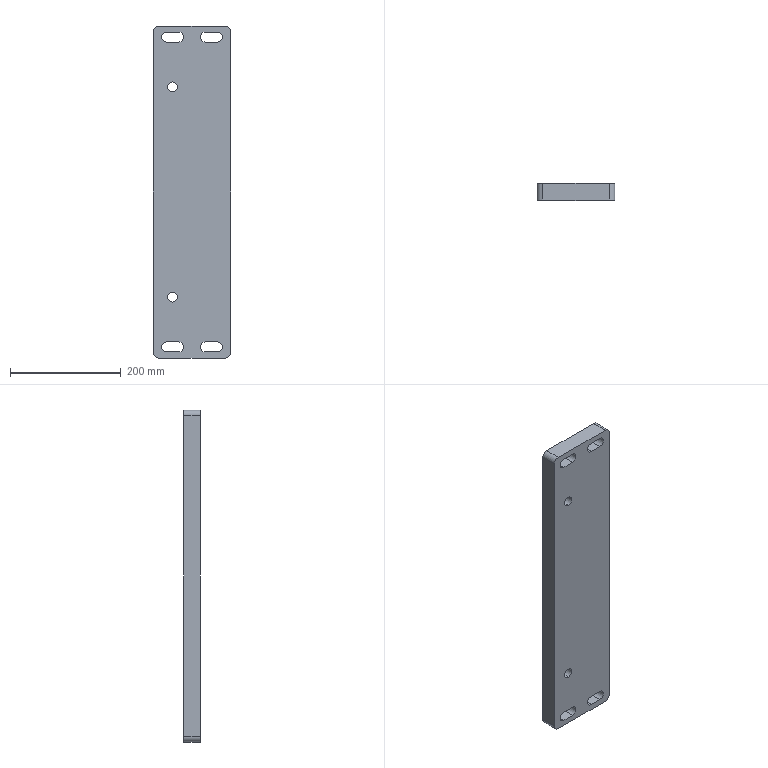Part | SolidWorks | features BaseBody 1 | 1 solid | 30 faces | box 140 x 30 x 600 mm | volume 2424100 mm3 | cylinder 16 | plane 14 | commonest cylinder face diameters 18 x12 20 x4
STEP:
#1=CARTESIAN_POINT('',(-35.,0.,181.));
#2=VERTEX_POINT('',#1);
#3=CARTESIAN_POINT('',(-35.,0.,199.));
#4=VERTEX_POINT('',#3);
#5=CARTESIAN_POINT('',(-35.,0.,190.));
#6=DIRECTION('',(0.,1.,0.));
#7=DIRECTION('',(0.,0.,1.));
#8=AXIS2_PLACEMENT_3D('',#5,#6,#7);
#9=CIRCLE('',#8,9.);
#10=EDGE_CURVE('',#2,#4,#9,.T.);
#11=ORIENTED_EDGE('',*,*,#10,.F.);
#12=CARTESIAN_POINT('',(-35.,30.,181.));
#13=VERTEX_POINT('',#12);
#14=CARTESIAN_POINT('',(-35.,30.,181.));
#15=DIRECTION('',(0.,1.,0.));
#16=VECTOR('',#15,1000.);
#17=LINE('',#14,#16);
#18=EDGE_CURVE('',#2,#13,#17,.T.);
#19=ORIENTED_EDGE('',*,*,#18,.T.);
#20=CARTESIAN_POINT('',(-35.,30.,199.));
#21=VERTEX_POINT('',#20);
#22=CARTESIAN_POINT('',(-35.,30.,190.));
#23=DIRECTION('',(0.,1.,0.));
#24=DIRECTION('',(0.,0.,1.));
#25=AXIS2_PLACEMENT_3D('',#22,#23,#24);
#26=CIRCLE('',#25,9.);
#27=EDGE_CURVE('',#13,#21,#26,.T.);
#28=ORIENTED_EDGE('',*,*,#27,.T.);
#29=CARTESIAN_POINT('',(-35.,30.,199.));
#30=DIRECTION('',(0.,1.,0.));
#31=VECTOR('',#30,1000.);
#32=LINE('',#29,#31);
#33=EDGE_CURVE('',#4,#21,#32,.T.);
#34=ORIENTED_EDGE('',*,*,#33,.F.);
#35=EDGE_LOOP('',(#11,#19,#28,#34));
#36=FACE_OUTER_BOUND('',#35,.T.);
#37=CARTESIAN_POINT('',(-35.,30.,190.));
#38=DIRECTION('',(0.,1.,0.));
#39=DIRECTION('',(0.,0.,1.));
#40=AXIS2_PLACEMENT_3D('',#37,#38,#39);
#41=CYLINDRICAL_SURFACE('',#40,9.);
#42=ADVANCED_FACE('',(#36),#41,.F.);
#43=CARTESIAN_POINT('',(-35.,0.,-199.));
#44=VERTEX_POINT('',#43);
#45=CARTESIAN_POINT('',(-35.,0.,-181.));
#46=VERTEX_POINT('',#45);
#47=CARTESIAN_POINT('',(-35.,0.,-190.));
#48=DIRECTION('',(0.,1.,0.));
#49=DIRECTION('',(0.,0.,1.));
#50=AXIS2_PLACEMENT_3D('',#47,#48,#49);
#51=CIRCLE('',#50,9.);
#52=EDGE_CURVE('',#44,#46,#51,.T.);
#53=ORIENTED_EDGE('',*,*,#52,.F.);
#54=CARTESIAN_POINT('',(-35.,30.,-199.));
#55=VERTEX_POINT('',#54);
#56=CARTESIAN_POINT('',(-35.,30.,-199.));
#57=DIRECTION('',(0.,1.,0.));
#58=VECTOR('',#57,1000.);
#59=LINE('',#56,#58);
#60=EDGE_CURVE('',#44,#55,#59,.T.);
#61=ORIENTED_EDGE('',*,*,#60,.T.);
#62=CARTESIAN_POINT('',(-35.,30.,-181.));
#63=VERTEX_POINT('',#62);
#64=CARTESIAN_POINT('',(-35.,30.,-190.));
#65=DIRECTION('',(0.,1.,0.));
#66=DIRECTION('',(0.,0.,1.));
#67=AXIS2_PLACEMENT_3D('',#64,#65,#66);
#68=CIRCLE('',#67,9.);
#69=EDGE_CURVE('',#55,#63,#68,.T.);
#70=ORIENTED_EDGE('',*,*,#69,.T.);
#71=CARTESIAN_POINT('',(-35.,30.,-181.));
#72=DIRECTION('',(0.,1.,0.));
#73=VECTOR('',#72,1000.);
#74=LINE('',#71,#73);
#75=EDGE_CURVE('',#46,#63,#74,.T.);
#76=ORIENTED_EDGE('',*,*,#75,.F.);
#77=EDGE_LOOP('',(#53,#61,#70,#76));
#78=FACE_OUTER_BOUND('',#77,.T.);
#79=CARTESIAN_POINT('',(-35.,30.,-190.));
#80=DIRECTION('',(0.,1.,0.));
#81=DIRECTION('',(0.,0.,1.));
#82=AXIS2_PLACEMENT_3D('',#79,#80,#81);
#83=CYLINDRICAL_SURFACE('',#82,9.);
#84=ADVANCED_FACE('',(#78),#83,.F.);
#85=CARTESIAN_POINT('',(70.,0.,290.));
#86=VERTEX_POINT('',#85);
#87=CARTESIAN_POINT('',(70.,0.,-290.));
#88=VERTEX_POINT('',#87);
#89=CARTESIAN_POINT('',(70.,0.,-300.));
#90=DIRECTION('',(0.,0.,-1.));
#91=VECTOR('',#90,1000.);
#92=LINE('',#89,#91);
#93=EDGE_CURVE('',#86,#88,#92,.T.);
#94=ORIENTED_EDGE('',*,*,#93,.T.);
#95=CARTESIAN_POINT('',(70.,30.,-290.));
#96=VERTEX_POINT('',#95);
#97=CARTESIAN_POINT('',(70.,30.,-290.));
#98=DIRECTION('',(0.,1.,0.));
#99=VECTOR('',#98,1000.);
#100=LINE('',#97,#99);
#101=EDGE_CURVE('',#88,#96,#100,.T.);
#102=ORIENTED_EDGE('',*,*,#101,.T.);
#103=CARTESIAN_POINT('',(70.,30.,290.));
#104=VERTEX_POINT('',#103);
#105=CARTESIAN_POINT('',(70.,30.,-300.));
#106=DIRECTION('',(0.,0.,-1.));
#107=VECTOR('',#106,1000.);
#108=LINE('',#105,#107);
#109=EDGE_CURVE('',#104,#96,#108,.T.);
#110=ORIENTED_EDGE('',*,*,#109,.F.);
#111=CARTESIAN_POINT('',(70.,30.,290.));
#112=DIRECTION('',(0.,-1.,0.));
#113=VECTOR('',#112,1000.);
#114=LINE('',#111,#113);
#115=EDGE_CURVE('',#104,#86,#114,.T.);
#116=ORIENTED_EDGE('',*,*,#115,.T.);
#117=EDGE_LOOP('',(#94,#102,#110,#116));
#118=FACE_OUTER_BOUND('',#117,.T.);
#119=CARTESIAN_POINT('',(70.,30.,-300.));
#120=DIRECTION('',(-1.,0.,0.));
#121=DIRECTION('',(0.,0.,1.));
#122=AXIS2_PLACEMENT_3D('',#119,#120,#121);
#123=PLANE('',#122);
#124=ADVANCED_FACE('',(#118),#123,.F.);
#125=CARTESIAN_POINT('',(60.,30.,-300.));
#126=VERTEX_POINT('',#125);
#127=CARTESIAN_POINT('',(-60.,30.,-300.));
#128=VERTEX_POINT('',#127);
#129=CARTESIAN_POINT('',(-70.,30.,-300.));
#130=DIRECTION('',(-1.,0.,0.));
#131=VECTOR('',#130,1000.);
#132=LINE('',#129,#131);
#133=EDGE_CURVE('',#126,#128,#132,.T.);
#134=ORIENTED_EDGE('',*,*,#133,.F.);
#135=CARTESIAN_POINT('',(60.,0.,-300.));
#136=VERTEX_POINT('',#135);
#137=CARTESIAN_POINT('',(60.,30.,-300.));
#138=DIRECTION('',(0.,-1.,0.));
#139=VECTOR('',#138,1000.);
#140=LINE('',#137,#139);
#141=EDGE_CURVE('',#126,#136,#140,.T.);
#142=ORIENTED_EDGE('',*,*,#141,.T.);
#143=CARTESIAN_POINT('',(-60.,0.,-300.));
#144=VERTEX_POINT('',#143);
#145=CARTESIAN_POINT('',(-70.,0.,-300.));
#146=DIRECTION('',(-1.,0.,0.));
#147=VECTOR('',#146,1000.);
#148=LINE('',#145,#147);
#149=EDGE_CURVE('',#136,#144,#148,.T.);
#150=ORIENTED_EDGE('',*,*,#149,.T.);
#151=CARTESIAN_POINT('',(-60.,30.,-300.));
#152=DIRECTION('',(0.,1.,0.));
#153=VECTOR('',#152,1000.);
#154=LINE('',#151,#153);
#155=EDGE_CURVE('',#144,#128,#154,.T.);
#156=ORIENTED_EDGE('',*,*,#155,.T.);
#157=EDGE_LOOP('',(#134,#142,#150,#156));
#158=FACE_OUTER_BOUND('',#157,.T.);
#159=CARTESIAN_POINT('',(-70.,30.,-300.));
#160=DIRECTION('',(0.,0.,1.));
#161=DIRECTION('',(1.,0.,0.));
#162=AXIS2_PLACEMENT_3D('',#159,#160,#161);
#163=PLANE('',#162);
#164=ADVANCED_FACE('',(#158),#163,.F.);
#165=CARTESIAN_POINT('',(-70.,30.,-290.));
#166=VERTEX_POINT('',#165);
#167=CARTESIAN_POINT('',(-70.,30.,290.));
#168=VERTEX_POINT('',#167);
#169=CARTESIAN_POINT('',(-70.,30.,-300.));
#170=DIRECTION('',(0.,0.,1.));
#171=VECTOR('',#170,1000.);
#172=LINE('',#169,#171);
#173=EDGE_CURVE('',#166,#168,#172,.T.);
#174=ORIENTED_EDGE('',*,*,#173,.F.);
#175=CARTESIAN_POINT('',(-70.,0.,-290.));
#176=VERTEX_POINT('',#175);
#177=CARTESIAN_POINT('',(-70.,30.,-290.));
#178=DIRECTION('',(0.,-1.,0.));
#179=VECTOR('',#178,1000.);
#180=LINE('',#177,#179);
#181=EDGE_CURVE('',#166,#176,#180,.T.);
#182=ORIENTED_EDGE('',*,*,#181,.T.);
#183=CARTESIAN_POINT('',(-70.,0.,290.));
#184=VERTEX_POINT('',#183);
#185=CARTESIAN_POINT('',(-70.,0.,-300.));
#186=DIRECTION('',(0.,0.,1.));
#187=VECTOR('',#186,1000.);
#188=LINE('',#185,#187);
#189=EDGE_CURVE('',#176,#184,#188,.T.);
#190=ORIENTED_EDGE('',*,*,#189,.T.);
#191=CARTESIAN_POINT('',(-70.,30.,290.));
#192=DIRECTION('',(0.,1.,0.));
#193=VECTOR('',#192,1000.);
#194=LINE('',#191,#193);
#195=EDGE_CURVE('',#184,#168,#194,.T.);
#196=ORIENTED_EDGE('',*,*,#195,.T.);
#197=EDGE_LOOP('',(#174,#182,#190,#196));
#198=FACE_OUTER_BOUND('',#197,.T.);
#199=CARTESIAN_POINT('',(-70.,30.,-300.));
#200=DIRECTION('',(1.,0.,0.));
#201=DIRECTION('',(0.,0.,-1.));
#202=AXIS2_PLACEMENT_3D('',#199,#200,#201);
#203=PLANE('',#202);
#204=ADVANCED_FACE('',(#198),#203,.F.);
#205=CARTESIAN_POINT('',(-60.,0.,300.));
#206=VERTEX_POINT('',#205);
#207=CARTESIAN_POINT('',(60.,0.,300.));
#208=VERTEX_POINT('',#207);
#209=CARTESIAN_POINT('',(-70.,0.,300.));
#210=DIRECTION('',(1.,0.,0.));
#211=VECTOR('',#210,1000.);
#212=LINE('',#209,#211);
#213=EDGE_CURVE('',#206,#208,#212,.T.);
#214=ORIENTED_EDGE('',*,*,#213,.T.);
#215=CARTESIAN_POINT('',(60.,30.,300.));
#216=VERTEX_POINT('',#215);
#217=CARTESIAN_POINT('',(60.,30.,300.));
#218=DIRECTION('',(0.,1.,0.));
#219=VECTOR('',#218,1000.);
#220=LINE('',#217,#219);
#221=EDGE_CURVE('',#208,#216,#220,.T.);
#222=ORIENTED_EDGE('',*,*,#221,.T.);
#223=CARTESIAN_POINT('',(-60.,30.,300.));
#224=VERTEX_POINT('',#223);
#225=CARTESIAN_POINT('',(-70.,30.,300.));
#226=DIRECTION('',(1.,0.,0.));
#227=VECTOR('',#226,1000.);
#228=LINE('',#225,#227);
#229=EDGE_CURVE('',#224,#216,#228,.T.);
#230=ORIENTED_EDGE('',*,*,#229,.F.);
#231=CARTESIAN_POINT('',(-60.,30.,300.));
#232=DIRECTION('',(0.,-1.,0.));
#233=VECTOR('',#232,1000.);
#234=LINE('',#231,#233);
#235=EDGE_CURVE('',#224,#206,#234,.T.);
#236=ORIENTED_EDGE('',*,*,#235,.T.);
#237=EDGE_LOOP('',(#214,#222,#230,#236));
#238=FACE_OUTER_BOUND('',#237,.T.);
#239=CARTESIAN_POINT('',(-70.,30.,300.));
#240=DIRECTION('',(0.,0.,-1.));
#241=DIRECTION('',(-1.,0.,0.));
#242=AXIS2_PLACEMENT_3D('',#239,#240,#241);
#243=PLANE('',#242);
#244=ADVANCED_FACE('',(#238),#243,.F.);
#245=CARTESIAN_POINT('',(24.,30.,271.));
#246=VERTEX_POINT('',#245);
#247=CARTESIAN_POINT('',(24.,30.,289.));
#248=VERTEX_POINT('',#247);
#249=CARTESIAN_POINT('',(24.,30.,280.));
#250=DIRECTION('',(0.,1.,0.));
#251=DIRECTION('',(0.,0.,1.));
#252=AXIS2_PLACEMENT_3D('',#249,#250,#251);
#253=CIRCLE('',#252,9.);
#254=EDGE_CURVE('',#246,#248,#253,.T.);
#255=ORIENTED_EDGE('',*,*,#254,.F.);
#256=CARTESIAN_POINT('',(46.,30.,271.));
#257=VERTEX_POINT('',#256);
#258=CARTESIAN_POINT('',(24.,30.,271.));
#259=DIRECTION('',(-1.,0.,0.));
#260=VECTOR('',#259,1000.);
#261=LINE('',#258,#260);
#262=EDGE_CURVE('',#257,#246,#261,.T.);
#263=ORIENTED_EDGE('',*,*,#262,.F.);
#264=CARTESIAN_POINT('',(46.,30.,289.));
#265=VERTEX_POINT('',#264);
#266=CARTESIAN_POINT('',(46.,30.,280.));
#267=DIRECTION('',(0.,1.,0.));
#268=DIRECTION('',(0.,0.,1.));
#269=AXIS2_PLACEMENT_3D('',#266,#267,#268);
#270=CIRCLE('',#269,9.);
#271=EDGE_CURVE('',#265,#257,#270,.T.);
#272=ORIENTED_EDGE('',*,*,#271,.F.);
#273=CARTESIAN_POINT('',(24.,30.,289.));
#274=DIRECTION('',(1.,0.,0.));
#275=VECTOR('',#274,1000.);
#276=LINE('',#273,#275);
#277=EDGE_CURVE('',#248,#265,#276,.T.);
#278=ORIENTED_EDGE('',*,*,#277,.F.);
#279=EDGE_LOOP('',(#255,#263,#272,#278));
#280=FACE_BOUND('',#279,.T.);
#281=CARTESIAN_POINT('',(-46.,30.,-289.));
#282=VERTEX_POINT('',#281);
#283=CARTESIAN_POINT('',(-46.,30.,-271.));
#284=VERTEX_POINT('',#283);
#285=CARTESIAN_POINT('',(-46.,30.,-280.));
#286=DIRECTION('',(0.,1.,0.));
#287=DIRECTION('',(0.,0.,-1.));
#288=AXIS2_PLACEMENT_3D('',#285,#286,#287);
#289=CIRCLE('',#288,9.);
#290=EDGE_CURVE('',#282,#284,#289,.T.);
#291=ORIENTED_EDGE('',*,*,#290,.F.);
#292=CARTESIAN_POINT('',(-24.,30.,-289.));
#293=VERTEX_POINT('',#292);
#294=CARTESIAN_POINT('',(-46.,30.,-289.));
#295=DIRECTION('',(-1.,0.,0.));
#296=VECTOR('',#295,1000.);
#297=LINE('',#294,#296);
#298=EDGE_CURVE('',#293,#282,#297,.T.);
#299=ORIENTED_EDGE('',*,*,#298,.F.);
#300=CARTESIAN_POINT('',(-24.,30.,-271.));
#301=VERTEX_POINT('',#300);
#302=CARTESIAN_POINT('',(-24.,30.,-280.));
#303=DIRECTION('',(0.,1.,0.));
#304=DIRECTION('',(0.,0.,-1.));
#305=AXIS2_PLACEMENT_3D('',#302,#303,#304);
#306=CIRCLE('',#305,9.);
#307=EDGE_CURVE('',#301,#293,#306,.T.);
#308=ORIENTED_EDGE('',*,*,#307,.F.);
#309=CARTESIAN_POINT('',(-46.,30.,-271.));
#310=DIRECTION('',(1.,0.,0.));
#311=VECTOR('',#310,1000.);
#312=LINE('',#309,#311);
#313=EDGE_CURVE('',#284,#301,#312,.T.);
#314=ORIENTED_EDGE('',*,*,#313,.F.);
#315=EDGE_LOOP('',(#291,#299,#308,#314));
#316=FACE_BOUND('',#315,.T.);
#317=CARTESIAN_POINT('',(24.,30.,-289.));
#318=VERTEX_POINT('',#317);
#319=CARTESIAN_POINT('',(24.,30.,-271.));
#320=VERTEX_POINT('',#319);
#321=CARTESIAN_POINT('',(24.,30.,-280.));
#322=DIRECTION('',(0.,1.,0.));
#323=DIRECTION('',(0.,0.,-1.));
#324=AXIS2_PLACEMENT_3D('',#321,#322,#323);
#325=CIRCLE('',#324,9.);
#326=EDGE_CURVE('',#318,#320,#325,.T.);
#327=ORIENTED_EDGE('',*,*,#326,.F.);
#328=CARTESIAN_POINT('',(46.,30.,-289.));
#329=VERTEX_POINT('',#328);
#330=CARTESIAN_POINT('',(24.,30.,-289.));
#331=DIRECTION('',(-1.,0.,0.));
#332=VECTOR('',#331,1000.);
#333=LINE('',#330,#332);
#334=EDGE_CURVE('',#329,#318,#333,.T.);
#335=ORIENTED_EDGE('',*,*,#334,.F.);
#336=CARTESIAN_POINT('',(46.,30.,-271.));
#337=VERTEX_POINT('',#336);
#338=CARTESIAN_POINT('',(46.,30.,-280.));
#339=DIRECTION('',(0.,1.,0.));
#340=DIRECTION('',(0.,0.,-1.));
#341=AXIS2_PLACEMENT_3D('',#338,#339,#340);
#342=CIRCLE('',#341,9.);
#343=EDGE_CURVE('',#337,#329,#342,.T.);
#344=ORIENTED_EDGE('',*,*,#343,.F.);
#345=CARTESIAN_POINT('',(24.,30.,-271.));
#346=DIRECTION('',(1.,0.,0.));
#347=VECTOR('',#346,1000.);
#348=LINE('',#345,#347);
#349=EDGE_CURVE('',#320,#337,#348,.T.);
#350=ORIENTED_EDGE('',*,*,#349,.F.);
#351=EDGE_LOOP('',(#327,#335,#344,#350));
#352=FACE_BOUND('',#351,.T.);
#353=CARTESIAN_POINT('',(-46.,30.,271.));
#354=VERTEX_POINT('',#353);
#355=CARTESIAN_POINT('',(-46.,30.,289.));
#356=VERTEX_POINT('',#355);
#357=CARTESIAN_POINT('',(-46.,30.,280.));
#358=DIRECTION('',(0.,1.,0.));
#359=DIRECTION('',(0.,0.,1.));
#360=AXIS2_PLACEMENT_3D('',#357,#358,#359);
#361=CIRCLE('',#360,9.);
#362=EDGE_CURVE('',#354,#356,#361,.T.);
#363=ORIENTED_EDGE('',*,*,#362,.F.);
#364=CARTESIAN_POINT('',(-24.,30.,271.));
#365=VERTEX_POINT('',#364);
#366=CARTESIAN_POINT('',(-46.,30.,271.));
#367=DIRECTION('',(-1.,0.,0.));
#368=VECTOR('',#367,1000.);
#369=LINE('',#366,#368);
#370=EDGE_CURVE('',#365,#354,#369,.T.);
#371=ORIENTED_EDGE('',*,*,#370,.F.);
#372=CARTESIAN_POINT('',(-24.,30.,289.));
#373=VERTEX_POINT('',#372);
#374=CARTESIAN_POINT('',(-24.,30.,280.));
#375=DIRECTION('',(0.,1.,0.));
#376=DIRECTION('',(0.,0.,1.));
#377=AXIS2_PLACEMENT_3D('',#374,#375,#376);
#378=CIRCLE('',#377,9.);
#379=EDGE_CURVE('',#373,#365,#378,.T.);
#380=ORIENTED_EDGE('',*,*,#379,.F.);
#381=CARTESIAN_POINT('',(-46.,30.,289.));
#382=DIRECTION('',(1.,0.,0.));
#383=VECTOR('',#382,1000.);
#384=LINE('',#381,#383);
#385=EDGE_CURVE('',#356,#373,#384,.T.);
#386=ORIENTED_EDGE('',*,*,#385,.F.);
#387=EDGE_LOOP('',(#363,#371,#380,#386));
#388=FACE_BOUND('',#387,.T.);
#389=CARTESIAN_POINT('',(-35.,30.,190.));
#390=DIRECTION('',(0.,1.,0.));
#391=DIRECTION('',(0.,0.,1.));
#392=AXIS2_PLACEMENT_3D('',#389,#390,#391);
#393=CIRCLE('',#392,9.);
#394=EDGE_CURVE('',#21,#13,#393,.T.);
#395=ORIENTED_EDGE('',*,*,#394,.F.);
#396=ORIENTED_EDGE('',*,*,#27,.F.);
#397=EDGE_LOOP('',(#395,#396));
#398=FACE_BOUND('',#397,.T.);
#399=CARTESIAN_POINT('',(-35.,30.,-190.));
#400=DIRECTION('',(0.,1.,0.));
#401=DIRECTION('',(0.,0.,1.));
#402=AXIS2_PLACEMENT_3D('',#399,#400,#401);
#403=CIRCLE('',#402,9.);
#404=EDGE_CURVE('',#63,#55,#403,.T.);
#405=ORIENTED_EDGE('',*,*,#404,.F.);
#406=ORIENTED_EDGE('',*,*,#69,.F.);
#407=EDGE_LOOP('',(#405,#406));
#408=FACE_BOUND('',#407,.T.);
#409=ORIENTED_EDGE('',*,*,#109,.T.);
#410=CARTESIAN_POINT('',(60.,30.,-290.));
#411=DIRECTION('',(0.,1.,0.));
#412=DIRECTION('',(0.,0.,1.));
#413=AXIS2_PLACEMENT_3D('',#410,#411,#412);
#414=CIRCLE('',#413,10.);
#415=EDGE_CURVE('',#96,#126,#414,.T.);
#416=ORIENTED_EDGE('',*,*,#415,.T.);
#417=ORIENTED_EDGE('',*,*,#133,.T.);
#418=CARTESIAN_POINT('',(-60.,30.,-290.));
#419=DIRECTION('',(0.,1.,0.));
#420=DIRECTION('',(0.,0.,1.));
#421=AXIS2_PLACEMENT_3D('',#418,#419,#420);
#422=CIRCLE('',#421,10.);
#423=EDGE_CURVE('',#128,#166,#422,.T.);
#424=ORIENTED_EDGE('',*,*,#423,.T.);
#425=ORIENTED_EDGE('',*,*,#173,.T.);
#426=CARTESIAN_POINT('',(-60.,30.,290.));
#427=DIRECTION('',(0.,1.,0.));
#428=DIRECTION('',(0.,0.,1.));
#429=AXIS2_PLACEMENT_3D('',#426,#427,#428);
#430=CIRCLE('',#429,10.);
#431=EDGE_CURVE('',#168,#224,#430,.T.);
#432=ORIENTED_EDGE('',*,*,#431,.T.);
#433=ORIENTED_EDGE('',*,*,#229,.T.);
#434=CARTESIAN_POINT('',(60.,30.,290.));
#435=DIRECTION('',(0.,1.,0.));
#436=DIRECTION('',(0.,0.,1.));
#437=AXIS2_PLACEMENT_3D('',#434,#435,#436);
#438=CIRCLE('',#437,10.);
#439=EDGE_CURVE('',#216,#104,#438,.T.);
#440=ORIENTED_EDGE('',*,*,#439,.T.);
#441=EDGE_LOOP('',(#409,#416,#417,#424,#425,#432,#433,#440));
#442=FACE_OUTER_BOUND('',#441,.T.);
#443=CARTESIAN_POINT('',(0.,30.,0.));
#444=DIRECTION('',(0.,1.,0.));
#445=DIRECTION('',(0.,0.,1.));
#446=AXIS2_PLACEMENT_3D('',#443,#444,#445);
#447=PLANE('',#446);
#448=ADVANCED_FACE('',(#280,#316,#352,#388,#398,#408,#442),#447,.T.);
#449=CARTESIAN_POINT('',(46.,0.,271.));
#450=VERTEX_POINT('',#449);
#451=CARTESIAN_POINT('',(24.,0.,271.));
#452=VERTEX_POINT('',#451);
#453=CARTESIAN_POINT('',(24.,0.,271.));
#454=DIRECTION('',(-1.,0.,0.));
#455=VECTOR('',#454,1000.);
#456=LINE('',#453,#455);
#457=EDGE_CURVE('',#450,#452,#456,.T.);
#458=ORIENTED_EDGE('',*,*,#457,.T.);
#459=CARTESIAN_POINT('',(24.,0.,289.));
#460=VERTEX_POINT('',#459);
#461=CARTESIAN_POINT('',(24.,0.,280.));
#462=DIRECTION('',(0.,1.,0.));
#463=DIRECTION('',(0.,0.,1.));
#464=AXIS2_PLACEMENT_3D('',#461,#462,#463);
#465=CIRCLE('',#464,9.);
#466=EDGE_CURVE('',#452,#460,#465,.T.);
#467=ORIENTED_EDGE('',*,*,#466,.T.);
#468=CARTESIAN_POINT('',(46.,0.,289.));
#469=VERTEX_POINT('',#468);
#470=CARTESIAN_POINT('',(24.,0.,289.));
#471=DIRECTION('',(1.,0.,0.));
#472=VECTOR('',#471,1000.);
#473=LINE('',#470,#472);
#474=EDGE_CURVE('',#460,#469,#473,.T.);
#475=ORIENTED_EDGE('',*,*,#474,.T.);
#476=CARTESIAN_POINT('',(46.,0.,280.));
#477=DIRECTION('',(0.,1.,0.));
#478=DIRECTION('',(0.,0.,1.));
#479=AXIS2_PLACEMENT_3D('',#476,#477,#478);
#480=CIRCLE('',#479,9.);
#481=EDGE_CURVE('',#469,#450,#480,.T.);
#482=ORIENTED_EDGE('',*,*,#481,.T.);
#483=EDGE_LOOP('',(#458,#467,#475,#482));
#484=FACE_BOUND('',#483,.T.);
#485=CARTESIAN_POINT('',(-24.,0.,-289.));
#486=VERTEX_POINT('',#485);
#487=CARTESIAN_POINT('',(-46.,0.,-289.));
#488=VERTEX_POINT('',#487);
#489=CARTESIAN_POINT('',(-46.,0.,-289.));
#490=DIRECTION('',(-1.,0.,0.));
#491=VECTOR('',#490,1000.);
#492=LINE('',#489,#491);
#493=EDGE_CURVE('',#486,#488,#492,.T.);
#494=ORIENTED_EDGE('',*,*,#493,.T.);
#495=CARTESIAN_POINT('',(-46.,0.,-271.));
#496=VERTEX_POINT('',#495);
#497=CARTESIAN_POINT('',(-46.,0.,-280.));
#498=DIRECTION('',(0.,1.,0.));
#499=DIRECTION('',(0.,0.,-1.));
#500=AXIS2_PLACEMENT_3D('',#497,#498,#499);
#501=CIRCLE('',#500,9.);
#502=EDGE_CURVE('',#488,#496,#501,.T.);
#503=ORIENTED_EDGE('',*,*,#502,.T.);
#504=CARTESIAN_POINT('',(-24.,0.,-271.));
#505=VERTEX_POINT('',#504);
#506=CARTESIAN_POINT('',(-46.,0.,-271.));
#507=DIRECTION('',(1.,0.,0.));
#508=VECTOR('',#507,1000.);
#509=LINE('',#506,#508);
#510=EDGE_CURVE('',#496,#505,#509,.T.);
#511=ORIENTED_EDGE('',*,*,#510,.T.);
#512=CARTESIAN_POINT('',(-24.,0.,-280.));
#513=DIRECTION('',(0.,1.,0.));
#514=DIRECTION('',(0.,0.,-1.));
#515=AXIS2_PLACEMENT_3D('',#512,#513,#514);
#516=CIRCLE('',#515,9.);
#517=EDGE_CURVE('',#505,#486,#516,.T.);
#518=ORIENTED_EDGE('',*,*,#517,.T.);
#519=EDGE_LOOP('',(#494,#503,#511,#518));
#520=FACE_BOUND('',#519,.T.);
#521=CARTESIAN_POINT('',(46.,0.,-289.));
#522=VERTEX_POINT('',#521);
#523=CARTESIAN_POINT('',(24.,0.,-289.));
#524=VERTEX_POINT('',#523);
#525=CARTESIAN_POINT('',(24.,0.,-289.));
#526=DIRECTION('',(-1.,0.,0.));
#527=VECTOR('',#526,1000.);
#528=LINE('',#525,#527);
#529=EDGE_CURVE('',#522,#524,#528,.T.);
#530=ORIENTED_EDGE('',*,*,#529,.T.);
#531=CARTESIAN_POINT('',(24.,0.,-271.));
#532=VERTEX_POINT('',#531);
#533=CARTESIAN_POINT('',(24.,0.,-280.));
#534=DIRECTION('',(0.,1.,0.));
#535=DIRECTION('',(0.,0.,-1.));
#536=AXIS2_PLACEMENT_3D('',#533,#534,#535);
#537=CIRCLE('',#536,9.);
#538=EDGE_CURVE('',#524,#532,#537,.T.);
#539=ORIENTED_EDGE('',*,*,#538,.T.);
#540=CARTESIAN_POINT('',(46.,0.,-271.));
#541=VERTEX_POINT('',#540);
#542=CARTESIAN_POINT('',(24.,0.,-271.));
#543=DIRECTION('',(1.,0.,0.));
#544=VECTOR('',#543,1000.);
#545=LINE('',#542,#544);
#546=EDGE_CURVE('',#532,#541,#545,.T.);
#547=ORIENTED_EDGE('',*,*,#546,.T.);
#548=CARTESIAN_POINT('',(46.,0.,-280.));
#549=DIRECTION('',(0.,1.,0.));
#550=DIRECTION('',(0.,0.,-1.));
#551=AXIS2_PLACEMENT_3D('',#548,#549,#550);
#552=CIRCLE('',#551,9.);
#553=EDGE_CURVE('',#541,#522,#552,.T.);
#554=ORIENTED_EDGE('',*,*,#553,.T.);
#555=EDGE_LOOP('',(#530,#539,#547,#554));
#556=FACE_BOUND('',#555,.T.);
#557=CARTESIAN_POINT('',(-24.,0.,271.));
#558=VERTEX_POINT('',#557);
#559=CARTESIAN_POINT('',(-46.,0.,271.));
#560=VERTEX_POINT('',#559);
#561=CARTESIAN_POINT('',(-46.,0.,271.));
#562=DIRECTION('',(-1.,0.,0.));
#563=VECTOR('',#562,1000.);
#564=LINE('',#561,#563);
#565=EDGE_CURVE('',#558,#560,#564,.T.);
#566=ORIENTED_EDGE('',*,*,#565,.T.);
#567=CARTESIAN_POINT('',(-46.,0.,289.));
#568=VERTEX_POINT('',#567);
#569=CARTESIAN_POINT('',(-46.,0.,280.));
#570=DIRECTION('',(0.,1.,0.));
#571=DIRECTION('',(0.,0.,1.));
#572=AXIS2_PLACEMENT_3D('',#569,#570,#571);
#573=CIRCLE('',#572,9.);
#574=EDGE_CURVE('',#560,#568,#573,.T.);
#575=ORIENTED_EDGE('',*,*,#574,.T.);
#576=CARTESIAN_POINT('',(-24.,0.,289.));
#577=VERTEX_POINT('',#576);
#578=CARTESIAN_POINT('',(-46.,0.,289.));
#579=DIRECTION('',(1.,0.,0.));
#580=VECTOR('',#579,1000.);
#581=LINE('',#578,#580);
#582=EDGE_CURVE('',#568,#577,#581,.T.);
#583=ORIENTED_EDGE('',*,*,#582,.T.);
#584=CARTESIAN_POINT('',(-24.,0.,280.));
#585=DIRECTION('',(0.,1.,0.));
#586=DIRECTION('',(0.,0.,1.));
#587=AXIS2_PLACEMENT_3D('',#584,#585,#586);
#588=CIRCLE('',#587,9.);
#589=EDGE_CURVE('',#577,#558,#588,.T.);
#590=ORIENTED_EDGE('',*,*,#589,.T.);
#591=EDGE_LOOP('',(#566,#575,#583,#590));
#592=FACE_BOUND('',#591,.T.);
#593=CARTESIAN_POINT('',(-35.,0.,190.));
#594=DIRECTION('',(0.,1.,0.));
#595=DIRECTION('',(0.,0.,1.));
#596=AXIS2_PLACEMENT_3D('',#593,#594,#595);
#597=CIRCLE('',#596,9.);
#598=EDGE_CURVE('',#4,#2,#597,.T.);
#599=ORIENTED_EDGE('',*,*,#598,.T.);
#600=ORIENTED_EDGE('',*,*,#10,.T.);
#601=EDGE_LOOP('',(#599,#600));
#602=FACE_BOUND('',#601,.T.);
#603=CARTESIAN_POINT('',(-35.,0.,-190.));
#604=DIRECTION('',(0.,1.,0.));
#605=DIRECTION('',(0.,0.,1.));
#606=AXIS2_PLACEMENT_3D('',#603,#604,#605);
#607=CIRCLE('',#606,9.);
#608=EDGE_CURVE('',#46,#44,#607,.T.);
#609=ORIENTED_EDGE('',*,*,#608,.T.);
#610=ORIENTED_EDGE('',*,*,#52,.T.);
#611=EDGE_LOOP('',(#609,#610));
#612=FACE_BOUND('',#611,.T.);
#613=ORIENTED_EDGE('',*,*,#149,.F.);
#614=CARTESIAN_POINT('',(60.,0.,-290.));
#615=DIRECTION('',(0.,-1.,0.));
#616=DIRECTION('',(0.,0.,1.));
#617=AXIS2_PLACEMENT_3D('',#614,#615,#616);
#618=CIRCLE('',#617,10.);
#619=EDGE_CURVE('',#136,#88,#618,.T.);
#620=ORIENTED_EDGE('',*,*,#619,.T.);
#621=ORIENTED_EDGE('',*,*,#93,.F.);
#622=CARTESIAN_POINT('',(60.,0.,290.));
#623=DIRECTION('',(0.,-1.,0.));
#624=DIRECTION('',(0.,0.,1.));
#625=AXIS2_PLACEMENT_3D('',#622,#623,#624);
#626=CIRCLE('',#625,10.);
#627=EDGE_CURVE('',#86,#208,#626,.T.);
#628=ORIENTED_EDGE('',*,*,#627,.T.);
#629=ORIENTED_EDGE('',*,*,#213,.F.);
#630=CARTESIAN_POINT('',(-60.,0.,290.));
#631=DIRECTION('',(0.,-1.,0.));
#632=DIRECTION('',(0.,0.,1.));
#633=AXIS2_PLACEMENT_3D('',#630,#631,#632);
#634=CIRCLE('',#633,10.);
#635=EDGE_CURVE('',#206,#184,#634,.T.);
#636=ORIENTED_EDGE('',*,*,#635,.T.);
#637=ORIENTED_EDGE('',*,*,#189,.F.);
#638=CARTESIAN_POINT('',(-60.,0.,-290.));
#639=DIRECTION('',(0.,-1.,0.));
#640=DIRECTION('',(0.,0.,1.));
#641=AXIS2_PLACEMENT_3D('',#638,#639,#640);
#642=CIRCLE('',#641,10.);
#643=EDGE_CURVE('',#176,#144,#642,.T.);
#644=ORIENTED_EDGE('',*,*,#643,.T.);
#645=EDGE_LOOP('',(#613,#620,#621,#628,#629,#636,#637,#644));
#646=FACE_OUTER_BOUND('',#645,.T.);
#647=CARTESIAN_POINT('',(0.,0.,0.));
#648=DIRECTION('',(0.,1.,0.));
#649=DIRECTION('',(0.,0.,1.));
#650=AXIS2_PLACEMENT_3D('',#647,#648,#649);
#651=PLANE('',#650);
#652=ADVANCED_FACE('',(#484,#520,#556,#592,#602,#612,#646),#651,.F.);
#653=ORIENTED_EDGE('',*,*,#60,.F.);
#654=ORIENTED_EDGE('',*,*,#608,.F.);
#655=ORIENTED_EDGE('',*,*,#75,.T.);
#656=ORIENTED_EDGE('',*,*,#404,.T.);
#657=EDGE_LOOP('',(#653,#654,#655,#656));
#658=FACE_OUTER_BOUND('',#657,.T.);
#659=CARTESIAN_POINT('',(-35.,30.,-190.));
#660=DIRECTION('',(0.,1.,0.));
#661=DIRECTION('',(0.,0.,1.));
#662=AXIS2_PLACEMENT_3D('',#659,#660,#661);
#663=CYLINDRICAL_SURFACE('',#662,9.);
#664=ADVANCED_FACE('',(#658),#663,.F.);
#665=ORIENTED_EDGE('',*,*,#18,.F.);
#666=ORIENTED_EDGE('',*,*,#598,.F.);
#667=ORIENTED_EDGE('',*,*,#33,.T.);
#668=ORIENTED_EDGE('',*,*,#394,.T.);
#669=EDGE_LOOP('',(#665,#666,#667,#668));
#670=FACE_OUTER_BOUND('',#669,.T.);
#671=CARTESIAN_POINT('',(-35.,30.,190.));
#672=DIRECTION('',(0.,1.,0.));
#673=DIRECTION('',(0.,0.,1.));
#674=AXIS2_PLACEMENT_3D('',#671,#672,#673);
#675=CYLINDRICAL_SURFACE('',#674,9.);
#676=ADVANCED_FACE('',(#670),#675,.F.);
#677=ORIENTED_EDGE('',*,*,#415,.F.);
#678=ORIENTED_EDGE('',*,*,#101,.F.);
#679=ORIENTED_EDGE('',*,*,#619,.F.);
#680=ORIENTED_EDGE('',*,*,#141,.F.);
#681=EDGE_LOOP('',(#677,#678,#679,#680));
#682=FACE_OUTER_BOUND('',#681,.T.);
#683=CARTESIAN_POINT('',(60.,30.,-290.));
#684=DIRECTION('',(0.,-1.,0.));
#685=DIRECTION('',(0.,0.,-1.));
#686=AXIS2_PLACEMENT_3D('',#683,#684,#685);
#687=CYLINDRICAL_SURFACE('',#686,10.);
#688=ADVANCED_FACE('',(#682),#687,.T.);
#689=ORIENTED_EDGE('',*,*,#423,.F.);
#690=ORIENTED_EDGE('',*,*,#155,.F.);
#691=ORIENTED_EDGE('',*,*,#643,.F.);
#692=ORIENTED_EDGE('',*,*,#181,.F.);
#693=EDGE_LOOP('',(#689,#690,#691,#692));
#694=FACE_OUTER_BOUND('',#693,.T.);
#695=CARTESIAN_POINT('',(-60.,30.,-290.));
#696=DIRECTION('',(0.,-1.,0.));
#697=DIRECTION('',(0.,0.,-1.));
#698=AXIS2_PLACEMENT_3D('',#695,#696,#697);
#699=CYLINDRICAL_SURFACE('',#698,10.);
#700=ADVANCED_FACE('',(#694),#699,.T.);
#701=ORIENTED_EDGE('',*,*,#439,.F.);
#702=ORIENTED_EDGE('',*,*,#221,.F.);
#703=ORIENTED_EDGE('',*,*,#627,.F.);
#704=ORIENTED_EDGE('',*,*,#115,.F.);
#705=EDGE_LOOP('',(#701,#702,#703,#704));
#706=FACE_OUTER_BOUND('',#705,.T.);
#707=CARTESIAN_POINT('',(60.,30.,290.));
#708=DIRECTION('',(0.,-1.,0.));
#709=DIRECTION('',(0.,0.,-1.));
#710=AXIS2_PLACEMENT_3D('',#707,#708,#709);
#711=CYLINDRICAL_SURFACE('',#710,10.);
#712=ADVANCED_FACE('',(#706),#711,.T.);
#713=ORIENTED_EDGE('',*,*,#431,.F.);
#714=ORIENTED_EDGE('',*,*,#195,.F.);
#715=ORIENTED_EDGE('',*,*,#635,.F.);
#716=ORIENTED_EDGE('',*,*,#235,.F.);
#717=EDGE_LOOP('',(#713,#714,#715,#716));
#718=FACE_OUTER_BOUND('',#717,.T.);
#719=CARTESIAN_POINT('',(-60.,30.,290.));
#720=DIRECTION('',(0.,-1.,0.));
#721=DIRECTION('',(0.,0.,-1.));
#722=AXIS2_PLACEMENT_3D('',#719,#720,#721);
#723=CYLINDRICAL_SURFACE('',#722,10.);
#724=ADVANCED_FACE('',(#718),#723,.T.);
#725=ORIENTED_EDGE('',*,*,#362,.T.);
#726=CARTESIAN_POINT('',(-46.,0.,289.));
#727=DIRECTION('',(0.,1.,0.));
#728=VECTOR('',#727,1000.);
#729=LINE('',#726,#728);
#730=EDGE_CURVE('',#568,#356,#729,.T.);
#731=ORIENTED_EDGE('',*,*,#730,.F.);
#732=ORIENTED_EDGE('',*,*,#574,.F.);
#733=CARTESIAN_POINT('',(-46.,0.,271.));
#734=DIRECTION('',(0.,1.,0.));
#735=VECTOR('',#734,1000.);
#736=LINE('',#733,#735);
#737=EDGE_CURVE('',#560,#354,#736,.T.);
#738=ORIENTED_EDGE('',*,*,#737,.T.);
#739=EDGE_LOOP('',(#725,#731,#732,#738));
#740=FACE_OUTER_BOUND('',#739,.T.);
#741=CARTESIAN_POINT('',(-46.,0.,280.));
#742=DIRECTION('',(0.,1.,0.));
#743=DIRECTION('',(0.,0.,1.));
#744=AXIS2_PLACEMENT_3D('',#741,#742,#743);
#745=CYLINDRICAL_SURFACE('',#744,9.);
#746=ADVANCED_FACE('',(#740),#745,.F.);
#747=ORIENTED_EDGE('',*,*,#370,.T.);
#748=ORIENTED_EDGE('',*,*,#737,.F.);
#749=ORIENTED_EDGE('',*,*,#565,.F.);
#750=CARTESIAN_POINT('',(-24.,0.,271.));
#751=DIRECTION('',(0.,1.,0.));
#752=VECTOR('',#751,1000.);
#753=LINE('',#750,#752);
#754=EDGE_CURVE('',#558,#365,#753,.T.);
#755=ORIENTED_EDGE('',*,*,#754,.T.);
#756=EDGE_LOOP('',(#747,#748,#749,#755));
#757=FACE_OUTER_BOUND('',#756,.T.);
#758=CARTESIAN_POINT('',(-46.,0.,271.));
#759=DIRECTION('',(0.,0.,-1.));
#760=DIRECTION('',(-1.,0.,0.));
#761=AXIS2_PLACEMENT_3D('',#758,#759,#760);
#762=PLANE('',#761);
#763=ADVANCED_FACE('',(#757),#762,.F.);
#764=ORIENTED_EDGE('',*,*,#379,.T.);
#765=ORIENTED_EDGE('',*,*,#754,.F.);
#766=ORIENTED_EDGE('',*,*,#589,.F.);
#767=CARTESIAN_POINT('',(-24.,0.,289.));
#768=DIRECTION('',(0.,1.,0.));
#769=VECTOR('',#768,1000.);
#770=LINE('',#767,#769);
#771=EDGE_CURVE('',#577,#373,#770,.T.);
#772=ORIENTED_EDGE('',*,*,#771,.T.);
#773=EDGE_LOOP('',(#764,#765,#766,#772));
#774=FACE_OUTER_BOUND('',#773,.T.);
#775=CARTESIAN_POINT('',(-24.,0.,280.));
#776=DIRECTION('',(0.,1.,0.));
#777=DIRECTION('',(0.,0.,1.));
#778=AXIS2_PLACEMENT_3D('',#775,#776,#777);
#779=CYLINDRICAL_SURFACE('',#778,9.);
#780=ADVANCED_FACE('',(#774),#779,.F.);
#781=ORIENTED_EDGE('',*,*,#385,.T.);
#782=ORIENTED_EDGE('',*,*,#771,.F.);
#783=ORIENTED_EDGE('',*,*,#582,.F.);
#784=ORIENTED_EDGE('',*,*,#730,.T.);
#785=EDGE_LOOP('',(#781,#782,#783,#784));
#786=FACE_OUTER_BOUND('',#785,.T.);
#787=CARTESIAN_POINT('',(-46.,0.,289.));
#788=DIRECTION('',(0.,0.,1.));
#789=DIRECTION('',(1.,0.,0.));
#790=AXIS2_PLACEMENT_3D('',#787,#788,#789);
#791=PLANE('',#790);
#792=ADVANCED_FACE('',(#786),#791,.F.);
#793=ORIENTED_EDGE('',*,*,#326,.T.);
#794=CARTESIAN_POINT('',(24.,0.,-271.));
#795=DIRECTION('',(0.,1.,0.));
#796=VECTOR('',#795,1000.);
#797=LINE('',#794,#796);
#798=EDGE_CURVE('',#532,#320,#797,.T.);
#799=ORIENTED_EDGE('',*,*,#798,.F.);
#800=ORIENTED_EDGE('',*,*,#538,.F.);
#801=CARTESIAN_POINT('',(24.,0.,-289.));
#802=DIRECTION('',(0.,1.,0.));
#803=VECTOR('',#802,1000.);
#804=LINE('',#801,#803);
#805=EDGE_CURVE('',#524,#318,#804,.T.);
#806=ORIENTED_EDGE('',*,*,#805,.T.);
#807=EDGE_LOOP('',(#793,#799,#800,#806));
#808=FACE_OUTER_BOUND('',#807,.T.);
#809=CARTESIAN_POINT('',(24.,0.,-280.));
#810=DIRECTION('',(0.,1.,0.));
#811=DIRECTION('',(0.,0.,1.));
#812=AXIS2_PLACEMENT_3D('',#809,#810,#811);
#813=CYLINDRICAL_SURFACE('',#812,9.);
#814=ADVANCED_FACE('',(#808),#813,.F.);
#815=ORIENTED_EDGE('',*,*,#334,.T.);
#816=ORIENTED_EDGE('',*,*,#805,.F.);
#817=ORIENTED_EDGE('',*,*,#529,.F.);
#818=CARTESIAN_POINT('',(46.,0.,-289.));
#819=DIRECTION('',(0.,1.,0.));
#820=VECTOR('',#819,1000.);
#821=LINE('',#818,#820);
#822=EDGE_CURVE('',#522,#329,#821,.T.);
#823=ORIENTED_EDGE('',*,*,#822,.T.);
#824=EDGE_LOOP('',(#815,#816,#817,#823));
#825=FACE_OUTER_BOUND('',#824,.T.);
#826=CARTESIAN_POINT('',(24.,0.,-289.));
#827=DIRECTION('',(0.,0.,-1.));
#828=DIRECTION('',(-1.,0.,0.));
#829=AXIS2_PLACEMENT_3D('',#826,#827,#828);
#830=PLANE('',#829);
#831=ADVANCED_FACE('',(#825),#830,.F.);
#832=ORIENTED_EDGE('',*,*,#343,.T.);
#833=ORIENTED_EDGE('',*,*,#822,.F.);
#834=ORIENTED_EDGE('',*,*,#553,.F.);
#835=CARTESIAN_POINT('',(46.,0.,-271.));
#836=DIRECTION('',(0.,1.,0.));
#837=VECTOR('',#836,1000.);
#838=LINE('',#835,#837);
#839=EDGE_CURVE('',#541,#337,#838,.T.);
#840=ORIENTED_EDGE('',*,*,#839,.T.);
#841=EDGE_LOOP('',(#832,#833,#834,#840));
#842=FACE_OUTER_BOUND('',#841,.T.);
#843=CARTESIAN_POINT('',(46.,0.,-280.));
#844=DIRECTION('',(0.,1.,0.));
#845=DIRECTION('',(0.,0.,1.));
#846=AXIS2_PLACEMENT_3D('',#843,#844,#845);
#847=CYLINDRICAL_SURFACE('',#846,9.);
#848=ADVANCED_FACE('',(#842),#847,.F.);
#849=ORIENTED_EDGE('',*,*,#349,.T.);
#850=ORIENTED_EDGE('',*,*,#839,.F.);
#851=ORIENTED_EDGE('',*,*,#546,.F.);
#852=ORIENTED_EDGE('',*,*,#798,.T.);
#853=EDGE_LOOP('',(#849,#850,#851,#852));
#854=FACE_OUTER_BOUND('',#853,.T.);
#855=CARTESIAN_POINT('',(24.,0.,-271.));
#856=DIRECTION('',(0.,0.,1.));
#857=DIRECTION('',(1.,0.,0.));
#858=AXIS2_PLACEMENT_3D('',#855,#856,#857);
#859=PLANE('',#858);
#860=ADVANCED_FACE('',(#854),#859,.F.);
#861=ORIENTED_EDGE('',*,*,#290,.T.);
#862=CARTESIAN_POINT('',(-46.,0.,-271.));
#863=DIRECTION('',(0.,1.,0.));
#864=VECTOR('',#863,1000.);
#865=LINE('',#862,#864);
#866=EDGE_CURVE('',#496,#284,#865,.T.);
#867=ORIENTED_EDGE('',*,*,#866,.F.);
#868=ORIENTED_EDGE('',*,*,#502,.F.);
#869=CARTESIAN_POINT('',(-46.,0.,-289.));
#870=DIRECTION('',(0.,1.,0.));
#871=VECTOR('',#870,1000.);
#872=LINE('',#869,#871);
#873=EDGE_CURVE('',#488,#282,#872,.T.);
#874=ORIENTED_EDGE('',*,*,#873,.T.);
#875=EDGE_LOOP('',(#861,#867,#868,#874));
#876=FACE_OUTER_BOUND('',#875,.T.);
#877=CARTESIAN_POINT('',(-46.,0.,-280.));
#878=DIRECTION('',(0.,1.,0.));
#879=DIRECTION('',(0.,0.,1.));
#880=AXIS2_PLACEMENT_3D('',#877,#878,#879);
#881=CYLINDRICAL_SURFACE('',#880,9.);
#882=ADVANCED_FACE('',(#876),#881,.F.);
#883=ORIENTED_EDGE('',*,*,#298,.T.);
#884=ORIENTED_EDGE('',*,*,#873,.F.);
#885=ORIENTED_EDGE('',*,*,#493,.F.);
#886=CARTESIAN_POINT('',(-24.,0.,-289.));
#887=DIRECTION('',(0.,1.,0.));
#888=VECTOR('',#887,1000.);
#889=LINE('',#886,#888);
#890=EDGE_CURVE('',#486,#293,#889,.T.);
#891=ORIENTED_EDGE('',*,*,#890,.T.);
#892=EDGE_LOOP('',(#883,#884,#885,#891));
#893=FACE_OUTER_BOUND('',#892,.T.);
#894=CARTESIAN_POINT('',(-46.,0.,-289.));
#895=DIRECTION('',(0.,0.,-1.));
#896=DIRECTION('',(-1.,0.,0.));
#897=AXIS2_PLACEMENT_3D('',#894,#895,#896);
#898=PLANE('',#897);
#899=ADVANCED_FACE('',(#893),#898,.F.);
#900=ORIENTED_EDGE('',*,*,#307,.T.);
#901=ORIENTED_EDGE('',*,*,#890,.F.);
#902=ORIENTED_EDGE('',*,*,#517,.F.);
#903=CARTESIAN_POINT('',(-24.,0.,-271.));
#904=DIRECTION('',(0.,1.,0.));
#905=VECTOR('',#904,1000.);
#906=LINE('',#903,#905);
#907=EDGE_CURVE('',#505,#301,#906,.T.);
#908=ORIENTED_EDGE('',*,*,#907,.T.);
#909=EDGE_LOOP('',(#900,#901,#902,#908));
#910=FACE_OUTER_BOUND('',#909,.T.);
#911=CARTESIAN_POINT('',(-24.,0.,-280.));
#912=DIRECTION('',(0.,1.,0.));
#913=DIRECTION('',(0.,0.,1.));
#914=AXIS2_PLACEMENT_3D('',#911,#912,#913);
#915=CYLINDRICAL_SURFACE('',#914,9.);
#916=ADVANCED_FACE('',(#910),#915,.F.);
#917=ORIENTED_EDGE('',*,*,#313,.T.);
#918=ORIENTED_EDGE('',*,*,#907,.F.);
#919=ORIENTED_EDGE('',*,*,#510,.F.);
#920=ORIENTED_EDGE('',*,*,#866,.T.);
#921=EDGE_LOOP('',(#917,#918,#919,#920));
#922=FACE_OUTER_BOUND('',#921,.T.);
#923=CARTESIAN_POINT('',(-46.,0.,-271.));
#924=DIRECTION('',(0.,0.,1.));
#925=DIRECTION('',(1.,0.,0.));
#926=AXIS2_PLACEMENT_3D('',#923,#924,#925);
#927=PLANE('',#926);
#928=ADVANCED_FACE('',(#922),#927,.F.);
#929=ORIENTED_EDGE('',*,*,#254,.T.);
#930=CARTESIAN_POINT('',(24.,0.,289.));
#931=DIRECTION('',(0.,1.,0.));
#932=VECTOR('',#931,1000.);
#933=LINE('',#930,#932);
#934=EDGE_CURVE('',#460,#248,#933,.T.);
#935=ORIENTED_EDGE('',*,*,#934,.F.);
#936=ORIENTED_EDGE('',*,*,#466,.F.);
#937=CARTESIAN_POINT('',(24.,0.,271.));
#938=DIRECTION('',(0.,1.,0.));
#939=VECTOR('',#938,1000.);
#940=LINE('',#937,#939);
#941=EDGE_CURVE('',#452,#246,#940,.T.);
#942=ORIENTED_EDGE('',*,*,#941,.T.);
#943=EDGE_LOOP('',(#929,#935,#936,#942));
#944=FACE_OUTER_BOUND('',#943,.T.);
#945=CARTESIAN_POINT('',(24.,0.,280.));
#946=DIRECTION('',(0.,1.,0.));
#947=DIRECTION('',(0.,0.,1.));
#948=AXIS2_PLACEMENT_3D('',#945,#946,#947);
#949=CYLINDRICAL_SURFACE('',#948,9.);
#950=ADVANCED_FACE('',(#944),#949,.F.);
#951=ORIENTED_EDGE('',*,*,#262,.T.);
#952=ORIENTED_EDGE('',*,*,#941,.F.);
#953=ORIENTED_EDGE('',*,*,#457,.F.);
#954=CARTESIAN_POINT('',(46.,0.,271.));
#955=DIRECTION('',(0.,1.,0.));
#956=VECTOR('',#955,1000.);
#957=LINE('',#954,#956);
#958=EDGE_CURVE('',#450,#257,#957,.T.);
#959=ORIENTED_EDGE('',*,*,#958,.T.);
#960=EDGE_LOOP('',(#951,#952,#953,#959));
#961=FACE_OUTER_BOUND('',#960,.T.);
#962=CARTESIAN_POINT('',(24.,0.,271.));
#963=DIRECTION('',(0.,0.,-1.));
#964=DIRECTION('',(-1.,0.,0.));
#965=AXIS2_PLACEMENT_3D('',#962,#963,#964);
#966=PLANE('',#965);
#967=ADVANCED_FACE('',(#961),#966,.F.);
#968=ORIENTED_EDGE('',*,*,#271,.T.);
#969=ORIENTED_EDGE('',*,*,#958,.F.);
#970=ORIENTED_EDGE('',*,*,#481,.F.);
#971=CARTESIAN_POINT('',(46.,0.,289.));
#972=DIRECTION('',(0.,1.,0.));
#973=VECTOR('',#972,1000.);
#974=LINE('',#971,#973);
#975=EDGE_CURVE('',#469,#265,#974,.T.);
#976=ORIENTED_EDGE('',*,*,#975,.T.);
#977=EDGE_LOOP('',(#968,#969,#970,#976));
#978=FACE_OUTER_BOUND('',#977,.T.);
#979=CARTESIAN_POINT('',(46.,0.,280.));
#980=DIRECTION('',(0.,1.,0.));
#981=DIRECTION('',(0.,0.,1.));
#982=AXIS2_PLACEMENT_3D('',#979,#980,#981);
#983=CYLINDRICAL_SURFACE('',#982,9.);
#984=ADVANCED_FACE('',(#978),#983,.F.);
#985=ORIENTED_EDGE('',*,*,#277,.T.);
#986=ORIENTED_EDGE('',*,*,#975,.F.);
#987=ORIENTED_EDGE('',*,*,#474,.F.);
#988=ORIENTED_EDGE('',*,*,#934,.T.);
#989=EDGE_LOOP('',(#985,#986,#987,#988));
#990=FACE_OUTER_BOUND('',#989,.T.);
#991=CARTESIAN_POINT('',(24.,0.,289.));
#992=DIRECTION('',(0.,0.,1.));
#993=DIRECTION('',(1.,0.,0.));
#994=AXIS2_PLACEMENT_3D('',#991,#992,#993);
#995=PLANE('',#994);
#996=ADVANCED_FACE('',(#990),#995,.F.);
#997=CLOSED_SHELL('',(#42,#84,#124,#164,#204,#244,#448,#652,#664,#676,#688,#700,#712,#724,#746,#763,#780,#792,#814,#831,#848,#860,#882,#899,#916,#928,#950,#967,#984,#996));
#998=MANIFOLD_SOLID_BREP('',#997);
#999=CARTESIAN_POINT('',(0.,0.,0.));
#1000=DIRECTION('',(0.,0.,1.));
#1001=DIRECTION('',(1.,0.,0.));
#1002=AXIS2_PLACEMENT_3D('',#999,#1000,#1001);
#1003=(LENGTH_UNIT()NAMED_UNIT(*)SI_UNIT(.MILLI.,.METRE.));
#1004=UNCERTAINTY_MEASURE_WITH_UNIT(LENGTH_MEASURE(0.00001),#1003,'','');
#1005=(NAMED_UNIT(*)PLANE_ANGLE_UNIT()SI_UNIT($,.RADIAN.));
#1006=(NAMED_UNIT(*)SI_UNIT($,.STERADIAN.)SOLID_ANGLE_UNIT());
#1007=(GEOMETRIC_REPRESENTATION_CONTEXT(3)GLOBAL_UNCERTAINTY_ASSIGNED_CONTEXT((#1004))GLOBAL_UNIT_ASSIGNED_CONTEXT((#1003,#1005,#1006))REPRESENTATION_CONTEXT('',''));
#1008=ADVANCED_BREP_SHAPE_REPRESENTATION('',(#998,#1002),#1007);